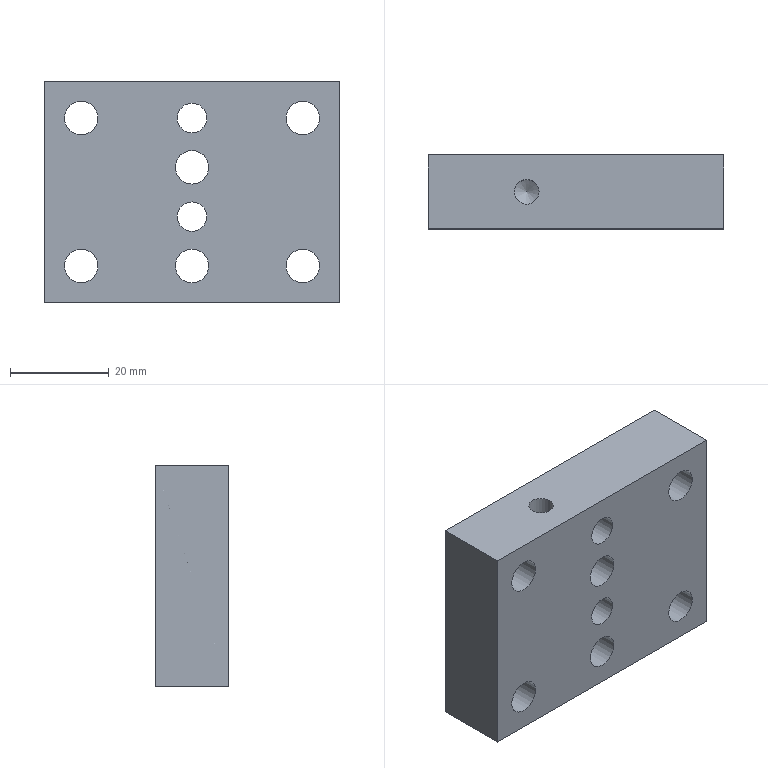Part | NX | features BREP 1 | 1 solid | 18 faces | box 60 x 15 x 45 mm | volume 35775 mm3 | cylinder 10 | plane 6 | cone 2 | commonest cylinder face diameters 6.8 x6 5 x2 6 x2
STEP:
#1=CARTESIAN_POINT('',(30.,0.,-2.5));
#2=VERTEX_POINT('',#1);
#3=CARTESIAN_POINT('',(30.,0.,0.));
#4=DIRECTION('',(1.,0.,0.));
#5=DIRECTION('',(0.,0.,-1.));
#6=AXIS2_PLACEMENT_3D('',#3,#4,#5);
#7=CIRCLE('',#6,2.5);
#8=EDGE_CURVE('',#2,#2,#7,.T.);
#9=ORIENTED_EDGE('',*,*,#8,.F.);
#10=EDGE_LOOP('',(#9));
#11=FACE_BOUND('',#10,.T.);
#12=CARTESIAN_POINT('',(30.,-7.5,22.5));
#13=VERTEX_POINT('',#12);
#14=CARTESIAN_POINT('',(30.,-7.5,-22.5));
#15=VERTEX_POINT('',#14);
#16=CARTESIAN_POINT('',(30.,-7.5,22.5));
#17=DIRECTION('',(0.,0.,-1.));
#18=VECTOR('',#17,1000.);
#19=LINE('',#16,#18);
#20=EDGE_CURVE('',#13,#15,#19,.T.);
#21=ORIENTED_EDGE('',*,*,#20,.T.);
#22=CARTESIAN_POINT('',(30.,7.5,-22.5));
#23=VERTEX_POINT('',#22);
#24=CARTESIAN_POINT('',(30.,7.5,-22.5));
#25=DIRECTION('',(0.,-1.,0.));
#26=VECTOR('',#25,1000.);
#27=LINE('',#24,#26);
#28=EDGE_CURVE('',#23,#15,#27,.T.);
#29=ORIENTED_EDGE('',*,*,#28,.F.);
#30=CARTESIAN_POINT('',(30.,7.5,22.5));
#31=VERTEX_POINT('',#30);
#32=CARTESIAN_POINT('',(30.,7.5,22.5));
#33=DIRECTION('',(0.,0.,-1.));
#34=VECTOR('',#33,1000.);
#35=LINE('',#32,#34);
#36=EDGE_CURVE('',#31,#23,#35,.T.);
#37=ORIENTED_EDGE('',*,*,#36,.F.);
#38=CARTESIAN_POINT('',(30.,7.5,22.5));
#39=DIRECTION('',(0.,-1.,0.));
#40=VECTOR('',#39,1000.);
#41=LINE('',#38,#40);
#42=EDGE_CURVE('',#31,#13,#41,.T.);
#43=ORIENTED_EDGE('',*,*,#42,.T.);
#44=EDGE_LOOP('',(#21,#29,#37,#43));
#45=FACE_BOUND('',#44,.T.);
#46=CARTESIAN_POINT('',(30.,7.5,22.5));
#47=DIRECTION('',(-1.,0.,0.));
#48=DIRECTION('',(0.,0.,-1.));
#49=AXIS2_PLACEMENT_3D('',#46,#47,#48);
#50=PLANE('',#49);
#51=ADVANCED_FACE('',(#11,#45),#50,.F.);
#52=CARTESIAN_POINT('',(-30.,-7.5,-22.5));
#53=VERTEX_POINT('',#52);
#54=CARTESIAN_POINT('',(-30.,-7.5,-22.5));
#55=DIRECTION('',(-1.,0.,0.));
#56=VECTOR('',#55,1000.);
#57=LINE('',#54,#56);
#58=EDGE_CURVE('',#15,#53,#57,.T.);
#59=ORIENTED_EDGE('',*,*,#58,.T.);
#60=CARTESIAN_POINT('',(-30.,7.5,-22.5));
#61=VERTEX_POINT('',#60);
#62=CARTESIAN_POINT('',(-30.,7.5,-22.5));
#63=DIRECTION('',(0.,-1.,0.));
#64=VECTOR('',#63,1000.);
#65=LINE('',#62,#64);
#66=EDGE_CURVE('',#61,#53,#65,.T.);
#67=ORIENTED_EDGE('',*,*,#66,.F.);
#68=CARTESIAN_POINT('',(-30.,7.5,-22.5));
#69=DIRECTION('',(-1.,0.,0.));
#70=VECTOR('',#69,1000.);
#71=LINE('',#68,#70);
#72=EDGE_CURVE('',#23,#61,#71,.T.);
#73=ORIENTED_EDGE('',*,*,#72,.F.);
#74=ORIENTED_EDGE('',*,*,#28,.T.);
#75=EDGE_LOOP('',(#59,#67,#73,#74));
#76=FACE_BOUND('',#75,.T.);
#77=CARTESIAN_POINT('',(-30.,7.5,-22.5));
#78=DIRECTION('',(0.,0.,1.));
#79=DIRECTION('',(-1.,0.,0.));
#80=AXIS2_PLACEMENT_3D('',#77,#78,#79);
#81=PLANE('',#80);
#82=ADVANCED_FACE('',(#76),#81,.F.);
#83=CARTESIAN_POINT('',(-30.,-7.5,22.5));
#84=VERTEX_POINT('',#83);
#85=CARTESIAN_POINT('',(-30.,-7.5,22.5));
#86=DIRECTION('',(0.,0.,1.));
#87=VECTOR('',#86,1000.);
#88=LINE('',#85,#87);
#89=EDGE_CURVE('',#53,#84,#88,.T.);
#90=ORIENTED_EDGE('',*,*,#89,.T.);
#91=CARTESIAN_POINT('',(-30.,7.5,22.5));
#92=VERTEX_POINT('',#91);
#93=CARTESIAN_POINT('',(-30.,7.5,22.5));
#94=DIRECTION('',(0.,-1.,0.));
#95=VECTOR('',#94,1000.);
#96=LINE('',#93,#95);
#97=EDGE_CURVE('',#92,#84,#96,.T.);
#98=ORIENTED_EDGE('',*,*,#97,.F.);
#99=CARTESIAN_POINT('',(-30.,7.5,22.5));
#100=DIRECTION('',(0.,0.,1.));
#101=VECTOR('',#100,1000.);
#102=LINE('',#99,#101);
#103=EDGE_CURVE('',#61,#92,#102,.T.);
#104=ORIENTED_EDGE('',*,*,#103,.F.);
#105=ORIENTED_EDGE('',*,*,#66,.T.);
#106=EDGE_LOOP('',(#90,#98,#104,#105));
#107=FACE_BOUND('',#106,.T.);
#108=CARTESIAN_POINT('',(-30.,7.5,22.5));
#109=DIRECTION('',(1.,0.,0.));
#110=DIRECTION('',(0.,0.,1.));
#111=AXIS2_PLACEMENT_3D('',#108,#109,#110);
#112=PLANE('',#111);
#113=ADVANCED_FACE('',(#107),#112,.F.);
#114=CARTESIAN_POINT('',(-7.5,0.,22.5));
#115=VERTEX_POINT('',#114);
#116=CARTESIAN_POINT('',(-10.,0.,22.5));
#117=DIRECTION('',(0.,0.,1.));
#118=DIRECTION('',(1.,0.,0.));
#119=AXIS2_PLACEMENT_3D('',#116,#117,#118);
#120=CIRCLE('',#119,2.5);
#121=EDGE_CURVE('',#115,#115,#120,.T.);
#122=ORIENTED_EDGE('',*,*,#121,.F.);
#123=EDGE_LOOP('',(#122));
#124=FACE_BOUND('',#123,.T.);
#125=CARTESIAN_POINT('',(-30.,-7.5,22.5));
#126=DIRECTION('',(1.,0.,0.));
#127=VECTOR('',#126,1000.);
#128=LINE('',#125,#127);
#129=EDGE_CURVE('',#84,#13,#128,.T.);
#130=ORIENTED_EDGE('',*,*,#129,.T.);
#131=ORIENTED_EDGE('',*,*,#42,.F.);
#132=CARTESIAN_POINT('',(-30.,7.5,22.5));
#133=DIRECTION('',(1.,0.,0.));
#134=VECTOR('',#133,1000.);
#135=LINE('',#132,#134);
#136=EDGE_CURVE('',#92,#31,#135,.T.);
#137=ORIENTED_EDGE('',*,*,#136,.F.);
#138=ORIENTED_EDGE('',*,*,#97,.T.);
#139=EDGE_LOOP('',(#130,#131,#137,#138));
#140=FACE_BOUND('',#139,.T.);
#141=CARTESIAN_POINT('',(-30.,7.5,22.5));
#142=DIRECTION('',(0.,0.,-1.));
#143=DIRECTION('',(1.,0.,0.));
#144=AXIS2_PLACEMENT_3D('',#141,#142,#143);
#145=PLANE('',#144);
#146=ADVANCED_FACE('',(#124,#140),#145,.F.);
#147=CARTESIAN_POINT('',(-22.5,7.5,-11.6));
#148=VERTEX_POINT('',#147);
#149=CARTESIAN_POINT('',(-22.5,7.5,-15.));
#150=DIRECTION('',(0.,1.,0.));
#151=DIRECTION('',(0.,0.,1.));
#152=AXIS2_PLACEMENT_3D('',#149,#150,#151);
#153=CIRCLE('',#152,3.4);
#154=EDGE_CURVE('',#148,#148,#153,.T.);
#155=ORIENTED_EDGE('',*,*,#154,.F.);
#156=EDGE_LOOP('',(#155));
#157=FACE_BOUND('',#156,.T.);
#158=CARTESIAN_POINT('',(22.5,7.5,18.4));
#159=VERTEX_POINT('',#158);
#160=CARTESIAN_POINT('',(22.5,7.5,15.));
#161=DIRECTION('',(0.,1.,0.));
#162=DIRECTION('',(0.,0.,1.));
#163=AXIS2_PLACEMENT_3D('',#160,#161,#162);
#164=CIRCLE('',#163,3.4);
#165=EDGE_CURVE('',#159,#159,#164,.T.);
#166=ORIENTED_EDGE('',*,*,#165,.F.);
#167=EDGE_LOOP('',(#166));
#168=FACE_BOUND('',#167,.T.);
#169=CARTESIAN_POINT('',(22.5,7.5,-11.6));
#170=VERTEX_POINT('',#169);
#171=CARTESIAN_POINT('',(22.5,7.5,-15.));
#172=DIRECTION('',(0.,1.,0.));
#173=DIRECTION('',(0.,0.,1.));
#174=AXIS2_PLACEMENT_3D('',#171,#172,#173);
#175=CIRCLE('',#174,3.4);
#176=EDGE_CURVE('',#170,#170,#175,.T.);
#177=ORIENTED_EDGE('',*,*,#176,.F.);
#178=EDGE_LOOP('',(#177));
#179=FACE_BOUND('',#178,.T.);
#180=CARTESIAN_POINT('',(-22.5,7.5,18.4));
#181=VERTEX_POINT('',#180);
#182=CARTESIAN_POINT('',(-22.5,7.5,15.));
#183=DIRECTION('',(0.,1.,0.));
#184=DIRECTION('',(0.,0.,1.));
#185=AXIS2_PLACEMENT_3D('',#182,#183,#184);
#186=CIRCLE('',#185,3.4);
#187=EDGE_CURVE('',#181,#181,#186,.T.);
#188=ORIENTED_EDGE('',*,*,#187,.F.);
#189=EDGE_LOOP('',(#188));
#190=FACE_BOUND('',#189,.T.);
#191=CARTESIAN_POINT('',(0.,7.5,8.4));
#192=VERTEX_POINT('',#191);
#193=CARTESIAN_POINT('',(0.,7.5,5.));
#194=DIRECTION('',(0.,1.,0.));
#195=DIRECTION('',(0.,0.,1.));
#196=AXIS2_PLACEMENT_3D('',#193,#194,#195);
#197=CIRCLE('',#196,3.4);
#198=EDGE_CURVE('',#192,#192,#197,.T.);
#199=ORIENTED_EDGE('',*,*,#198,.F.);
#200=EDGE_LOOP('',(#199));
#201=FACE_BOUND('',#200,.T.);
#202=CARTESIAN_POINT('',(0.,7.5,-11.6));
#203=VERTEX_POINT('',#202);
#204=CARTESIAN_POINT('',(0.,7.5,-15.));
#205=DIRECTION('',(0.,1.,0.));
#206=DIRECTION('',(0.,0.,1.));
#207=AXIS2_PLACEMENT_3D('',#204,#205,#206);
#208=CIRCLE('',#207,3.4);
#209=EDGE_CURVE('',#203,#203,#208,.T.);
#210=ORIENTED_EDGE('',*,*,#209,.F.);
#211=EDGE_LOOP('',(#210));
#212=FACE_BOUND('',#211,.T.);
#213=CARTESIAN_POINT('',(0.,7.5,-2.));
#214=VERTEX_POINT('',#213);
#215=CARTESIAN_POINT('',(0.,7.5,-5.));
#216=DIRECTION('',(0.,1.,0.));
#217=DIRECTION('',(0.,0.,1.));
#218=AXIS2_PLACEMENT_3D('',#215,#216,#217);
#219=CIRCLE('',#218,3.);
#220=EDGE_CURVE('',#214,#214,#219,.T.);
#221=ORIENTED_EDGE('',*,*,#220,.F.);
#222=EDGE_LOOP('',(#221));
#223=FACE_BOUND('',#222,.T.);
#224=CARTESIAN_POINT('',(0.,7.5,18.));
#225=VERTEX_POINT('',#224);
#226=CARTESIAN_POINT('',(0.,7.5,15.));
#227=DIRECTION('',(0.,1.,0.));
#228=DIRECTION('',(0.,0.,1.));
#229=AXIS2_PLACEMENT_3D('',#226,#227,#228);
#230=CIRCLE('',#229,3.);
#231=EDGE_CURVE('',#225,#225,#230,.T.);
#232=ORIENTED_EDGE('',*,*,#231,.F.);
#233=EDGE_LOOP('',(#232));
#234=FACE_BOUND('',#233,.T.);
#235=ORIENTED_EDGE('',*,*,#36,.T.);
#236=ORIENTED_EDGE('',*,*,#72,.T.);
#237=ORIENTED_EDGE('',*,*,#103,.T.);
#238=ORIENTED_EDGE('',*,*,#136,.T.);
#239=EDGE_LOOP('',(#235,#236,#237,#238));
#240=FACE_BOUND('',#239,.T.);
#241=CARTESIAN_POINT('',(0.,7.5,0.));
#242=DIRECTION('',(0.,-1.,0.));
#243=DIRECTION('',(0.,0.,1.));
#244=AXIS2_PLACEMENT_3D('',#241,#242,#243);
#245=PLANE('',#244);
#246=ADVANCED_FACE('',(#157,#168,#179,#190,#201,#212,#223,#234,#240),#245,.F.);
#247=CARTESIAN_POINT('',(-22.5,-7.5,-11.6));
#248=VERTEX_POINT('',#247);
#249=CARTESIAN_POINT('',(-22.5,-7.5,-15.));
#250=DIRECTION('',(0.,1.,0.));
#251=DIRECTION('',(0.,0.,1.));
#252=AXIS2_PLACEMENT_3D('',#249,#250,#251);
#253=CIRCLE('',#252,3.4);
#254=EDGE_CURVE('',#248,#248,#253,.T.);
#255=ORIENTED_EDGE('',*,*,#254,.T.);
#256=EDGE_LOOP('',(#255));
#257=FACE_BOUND('',#256,.T.);
#258=CARTESIAN_POINT('',(22.5,-7.5,18.4));
#259=VERTEX_POINT('',#258);
#260=CARTESIAN_POINT('',(22.5,-7.5,15.));
#261=DIRECTION('',(0.,1.,0.));
#262=DIRECTION('',(0.,0.,1.));
#263=AXIS2_PLACEMENT_3D('',#260,#261,#262);
#264=CIRCLE('',#263,3.4);
#265=EDGE_CURVE('',#259,#259,#264,.T.);
#266=ORIENTED_EDGE('',*,*,#265,.T.);
#267=EDGE_LOOP('',(#266));
#268=FACE_BOUND('',#267,.T.);
#269=CARTESIAN_POINT('',(22.5,-7.5,-11.6));
#270=VERTEX_POINT('',#269);
#271=CARTESIAN_POINT('',(22.5,-7.5,-15.));
#272=DIRECTION('',(0.,1.,0.));
#273=DIRECTION('',(0.,0.,1.));
#274=AXIS2_PLACEMENT_3D('',#271,#272,#273);
#275=CIRCLE('',#274,3.4);
#276=EDGE_CURVE('',#270,#270,#275,.T.);
#277=ORIENTED_EDGE('',*,*,#276,.T.);
#278=EDGE_LOOP('',(#277));
#279=FACE_BOUND('',#278,.T.);
#280=CARTESIAN_POINT('',(-22.5,-7.5,18.4));
#281=VERTEX_POINT('',#280);
#282=CARTESIAN_POINT('',(-22.5,-7.5,15.));
#283=DIRECTION('',(0.,1.,0.));
#284=DIRECTION('',(0.,0.,1.));
#285=AXIS2_PLACEMENT_3D('',#282,#283,#284);
#286=CIRCLE('',#285,3.4);
#287=EDGE_CURVE('',#281,#281,#286,.T.);
#288=ORIENTED_EDGE('',*,*,#287,.T.);
#289=EDGE_LOOP('',(#288));
#290=FACE_BOUND('',#289,.T.);
#291=CARTESIAN_POINT('',(0.,-7.5,8.4));
#292=VERTEX_POINT('',#291);
#293=CARTESIAN_POINT('',(0.,-7.5,5.));
#294=DIRECTION('',(0.,1.,0.));
#295=DIRECTION('',(0.,0.,1.));
#296=AXIS2_PLACEMENT_3D('',#293,#294,#295);
#297=CIRCLE('',#296,3.4);
#298=EDGE_CURVE('',#292,#292,#297,.T.);
#299=ORIENTED_EDGE('',*,*,#298,.T.);
#300=EDGE_LOOP('',(#299));
#301=FACE_BOUND('',#300,.T.);
#302=CARTESIAN_POINT('',(0.,-7.5,-11.6));
#303=VERTEX_POINT('',#302);
#304=CARTESIAN_POINT('',(0.,-7.5,-15.));
#305=DIRECTION('',(0.,1.,0.));
#306=DIRECTION('',(0.,0.,1.));
#307=AXIS2_PLACEMENT_3D('',#304,#305,#306);
#308=CIRCLE('',#307,3.4);
#309=EDGE_CURVE('',#303,#303,#308,.T.);
#310=ORIENTED_EDGE('',*,*,#309,.T.);
#311=EDGE_LOOP('',(#310));
#312=FACE_BOUND('',#311,.T.);
#313=CARTESIAN_POINT('',(0.,-7.5,-2.));
#314=VERTEX_POINT('',#313);
#315=CARTESIAN_POINT('',(0.,-7.5,-5.));
#316=DIRECTION('',(0.,1.,0.));
#317=DIRECTION('',(0.,0.,1.));
#318=AXIS2_PLACEMENT_3D('',#315,#316,#317);
#319=CIRCLE('',#318,3.);
#320=EDGE_CURVE('',#314,#314,#319,.T.);
#321=ORIENTED_EDGE('',*,*,#320,.T.);
#322=EDGE_LOOP('',(#321));
#323=FACE_BOUND('',#322,.T.);
#324=CARTESIAN_POINT('',(0.,-7.5,18.));
#325=VERTEX_POINT('',#324);
#326=CARTESIAN_POINT('',(0.,-7.5,15.));
#327=DIRECTION('',(0.,1.,0.));
#328=DIRECTION('',(0.,0.,1.));
#329=AXIS2_PLACEMENT_3D('',#326,#327,#328);
#330=CIRCLE('',#329,3.);
#331=EDGE_CURVE('',#325,#325,#330,.T.);
#332=ORIENTED_EDGE('',*,*,#331,.T.);
#333=EDGE_LOOP('',(#332));
#334=FACE_BOUND('',#333,.T.);
#335=ORIENTED_EDGE('',*,*,#20,.F.);
#336=ORIENTED_EDGE('',*,*,#129,.F.);
#337=ORIENTED_EDGE('',*,*,#89,.F.);
#338=ORIENTED_EDGE('',*,*,#58,.F.);
#339=EDGE_LOOP('',(#335,#336,#337,#338));
#340=FACE_BOUND('',#339,.T.);
#341=CARTESIAN_POINT('',(0.,-7.5,0.));
#342=DIRECTION('',(0.,-1.,0.));
#343=DIRECTION('',(0.,0.,1.));
#344=AXIS2_PLACEMENT_3D('',#341,#342,#343);
#345=PLANE('',#344);
#346=ADVANCED_FACE('',(#257,#268,#279,#290,#301,#312,#323,#334,#340),#345,.T.);
#347=CARTESIAN_POINT('',(13.498,0.,0.));
#348=VERTEX_POINT('',#347);
#349=VERTEX_LOOP('',#348);
#350=FACE_BOUND('',#349,.T.);
#351=CARTESIAN_POINT('',(15.,0.,-2.5));
#352=VERTEX_POINT('',#351);
#353=CARTESIAN_POINT('',(15.,0.,0.));
#354=DIRECTION('',(1.,0.,0.));
#355=DIRECTION('',(0.,0.,-1.));
#356=AXIS2_PLACEMENT_3D('',#353,#354,#355);
#357=CIRCLE('',#356,2.5);
#358=EDGE_CURVE('',#352,#352,#357,.T.);
#359=ORIENTED_EDGE('',*,*,#358,.T.);
#360=EDGE_LOOP('',(#359));
#361=FACE_BOUND('',#360,.T.);
#362=CARTESIAN_POINT('',(15.,0.,0.));
#363=DIRECTION('',(1.,0.,0.));
#364=DIRECTION('',(0.,0.,1.));
#365=AXIS2_PLACEMENT_3D('',#362,#363,#364);
#366=CONICAL_SURFACE('',#365,2.5,1.03);
#367=ADVANCED_FACE('',(#350,#361),#366,.F.);
#368=ORIENTED_EDGE('',*,*,#358,.F.);
#369=EDGE_LOOP('',(#368));
#370=FACE_BOUND('',#369,.T.);
#371=ORIENTED_EDGE('',*,*,#8,.T.);
#372=EDGE_LOOP('',(#371));
#373=FACE_BOUND('',#372,.T.);
#374=CARTESIAN_POINT('',(30.,0.,0.));
#375=DIRECTION('',(1.,0.,0.));
#376=DIRECTION('',(0.,0.,1.));
#377=AXIS2_PLACEMENT_3D('',#374,#375,#376);
#378=CYLINDRICAL_SURFACE('',#377,2.5);
#379=ADVANCED_FACE('',(#370,#373),#378,.F.);
#380=CARTESIAN_POINT('',(-10.,0.,5.998));
#381=VERTEX_POINT('',#380);
#382=VERTEX_LOOP('',#381);
#383=FACE_BOUND('',#382,.T.);
#384=CARTESIAN_POINT('',(-7.5,0.,7.5));
#385=VERTEX_POINT('',#384);
#386=CARTESIAN_POINT('',(-10.,0.,7.5));
#387=DIRECTION('',(0.,0.,1.));
#388=DIRECTION('',(1.,0.,0.));
#389=AXIS2_PLACEMENT_3D('',#386,#387,#388);
#390=CIRCLE('',#389,2.5);
#391=EDGE_CURVE('',#385,#385,#390,.T.);
#392=ORIENTED_EDGE('',*,*,#391,.T.);
#393=EDGE_LOOP('',(#392));
#394=FACE_BOUND('',#393,.T.);
#395=CARTESIAN_POINT('',(-10.,0.,7.5));
#396=DIRECTION('',(0.,0.,1.));
#397=DIRECTION('',(-1.,0.,0.));
#398=AXIS2_PLACEMENT_3D('',#395,#396,#397);
#399=CONICAL_SURFACE('',#398,2.5,1.03);
#400=ADVANCED_FACE('',(#383,#394),#399,.F.);
#401=ORIENTED_EDGE('',*,*,#391,.F.);
#402=EDGE_LOOP('',(#401));
#403=FACE_BOUND('',#402,.T.);
#404=ORIENTED_EDGE('',*,*,#121,.T.);
#405=EDGE_LOOP('',(#404));
#406=FACE_BOUND('',#405,.T.);
#407=CARTESIAN_POINT('',(-10.,0.,22.5));
#408=DIRECTION('',(0.,0.,1.));
#409=DIRECTION('',(-1.,0.,0.));
#410=AXIS2_PLACEMENT_3D('',#407,#408,#409);
#411=CYLINDRICAL_SURFACE('',#410,2.5);
#412=ADVANCED_FACE('',(#403,#406),#411,.F.);
#413=ORIENTED_EDGE('',*,*,#331,.F.);
#414=EDGE_LOOP('',(#413));
#415=FACE_BOUND('',#414,.T.);
#416=ORIENTED_EDGE('',*,*,#231,.T.);
#417=EDGE_LOOP('',(#416));
#418=FACE_BOUND('',#417,.T.);
#419=CARTESIAN_POINT('',(0.,7.5,15.));
#420=DIRECTION('',(0.,1.,0.));
#421=DIRECTION('',(0.,0.,-1.));
#422=AXIS2_PLACEMENT_3D('',#419,#420,#421);
#423=CYLINDRICAL_SURFACE('',#422,3.);
#424=ADVANCED_FACE('',(#415,#418),#423,.F.);
#425=ORIENTED_EDGE('',*,*,#320,.F.);
#426=EDGE_LOOP('',(#425));
#427=FACE_BOUND('',#426,.T.);
#428=ORIENTED_EDGE('',*,*,#220,.T.);
#429=EDGE_LOOP('',(#428));
#430=FACE_BOUND('',#429,.T.);
#431=CARTESIAN_POINT('',(0.,7.5,-5.));
#432=DIRECTION('',(0.,1.,0.));
#433=DIRECTION('',(0.,0.,-1.));
#434=AXIS2_PLACEMENT_3D('',#431,#432,#433);
#435=CYLINDRICAL_SURFACE('',#434,3.);
#436=ADVANCED_FACE('',(#427,#430),#435,.F.);
#437=ORIENTED_EDGE('',*,*,#309,.F.);
#438=EDGE_LOOP('',(#437));
#439=FACE_BOUND('',#438,.T.);
#440=ORIENTED_EDGE('',*,*,#209,.T.);
#441=EDGE_LOOP('',(#440));
#442=FACE_BOUND('',#441,.T.);
#443=CARTESIAN_POINT('',(0.,7.5,-15.));
#444=DIRECTION('',(0.,1.,0.));
#445=DIRECTION('',(0.,0.,-1.));
#446=AXIS2_PLACEMENT_3D('',#443,#444,#445);
#447=CYLINDRICAL_SURFACE('',#446,3.4);
#448=ADVANCED_FACE('',(#439,#442),#447,.F.);
#449=ORIENTED_EDGE('',*,*,#298,.F.);
#450=EDGE_LOOP('',(#449));
#451=FACE_BOUND('',#450,.T.);
#452=ORIENTED_EDGE('',*,*,#198,.T.);
#453=EDGE_LOOP('',(#452));
#454=FACE_BOUND('',#453,.T.);
#455=CARTESIAN_POINT('',(0.,7.5,5.));
#456=DIRECTION('',(0.,1.,0.));
#457=DIRECTION('',(0.,0.,-1.));
#458=AXIS2_PLACEMENT_3D('',#455,#456,#457);
#459=CYLINDRICAL_SURFACE('',#458,3.4);
#460=ADVANCED_FACE('',(#451,#454),#459,.F.);
#461=ORIENTED_EDGE('',*,*,#287,.F.);
#462=EDGE_LOOP('',(#461));
#463=FACE_BOUND('',#462,.T.);
#464=ORIENTED_EDGE('',*,*,#187,.T.);
#465=EDGE_LOOP('',(#464));
#466=FACE_BOUND('',#465,.T.);
#467=CARTESIAN_POINT('',(-22.5,7.5,15.));
#468=DIRECTION('',(0.,1.,0.));
#469=DIRECTION('',(0.,0.,-1.));
#470=AXIS2_PLACEMENT_3D('',#467,#468,#469);
#471=CYLINDRICAL_SURFACE('',#470,3.4);
#472=ADVANCED_FACE('',(#463,#466),#471,.F.);
#473=ORIENTED_EDGE('',*,*,#276,.F.);
#474=EDGE_LOOP('',(#473));
#475=FACE_BOUND('',#474,.T.);
#476=ORIENTED_EDGE('',*,*,#176,.T.);
#477=EDGE_LOOP('',(#476));
#478=FACE_BOUND('',#477,.T.);
#479=CARTESIAN_POINT('',(22.5,7.5,-15.));
#480=DIRECTION('',(0.,1.,0.));
#481=DIRECTION('',(0.,0.,-1.));
#482=AXIS2_PLACEMENT_3D('',#479,#480,#481);
#483=CYLINDRICAL_SURFACE('',#482,3.4);
#484=ADVANCED_FACE('',(#475,#478),#483,.F.);
#485=ORIENTED_EDGE('',*,*,#265,.F.);
#486=EDGE_LOOP('',(#485));
#487=FACE_BOUND('',#486,.T.);
#488=ORIENTED_EDGE('',*,*,#165,.T.);
#489=EDGE_LOOP('',(#488));
#490=FACE_BOUND('',#489,.T.);
#491=CARTESIAN_POINT('',(22.5,7.5,15.));
#492=DIRECTION('',(0.,1.,0.));
#493=DIRECTION('',(0.,0.,-1.));
#494=AXIS2_PLACEMENT_3D('',#491,#492,#493);
#495=CYLINDRICAL_SURFACE('',#494,3.4);
#496=ADVANCED_FACE('',(#487,#490),#495,.F.);
#497=ORIENTED_EDGE('',*,*,#254,.F.);
#498=EDGE_LOOP('',(#497));
#499=FACE_BOUND('',#498,.T.);
#500=ORIENTED_EDGE('',*,*,#154,.T.);
#501=EDGE_LOOP('',(#500));
#502=FACE_BOUND('',#501,.T.);
#503=CARTESIAN_POINT('',(-22.5,7.5,-15.));
#504=DIRECTION('',(0.,1.,0.));
#505=DIRECTION('',(0.,0.,-1.));
#506=AXIS2_PLACEMENT_3D('',#503,#504,#505);
#507=CYLINDRICAL_SURFACE('',#506,3.4);
#508=ADVANCED_FACE('',(#499,#502),#507,.F.);
#509=CLOSED_SHELL('',(#51,#82,#113,#146,#246,#346,#367,#379,#400,#412,#424,#436,#448,#460,#472,#484,#496,#508));
#510=MANIFOLD_SOLID_BREP('',#509);
#511=(LENGTH_UNIT()NAMED_UNIT(*)SI_UNIT(.MILLI.,.METRE.));
#512=UNCERTAINTY_MEASURE_WITH_UNIT(LENGTH_MEASURE(0.00001),#511,'','');
#513=(NAMED_UNIT(*)PLANE_ANGLE_UNIT()SI_UNIT($,.RADIAN.));
#514=(NAMED_UNIT(*)SI_UNIT($,.STERADIAN.)SOLID_ANGLE_UNIT());
#515=(GEOMETRIC_REPRESENTATION_CONTEXT(3)GLOBAL_UNCERTAINTY_ASSIGNED_CONTEXT((#512))GLOBAL_UNIT_ASSIGNED_CONTEXT((#511,#513,#514))REPRESENTATION_CONTEXT('',''));
#516=ADVANCED_BREP_SHAPE_REPRESENTATION('',(#510),#515);